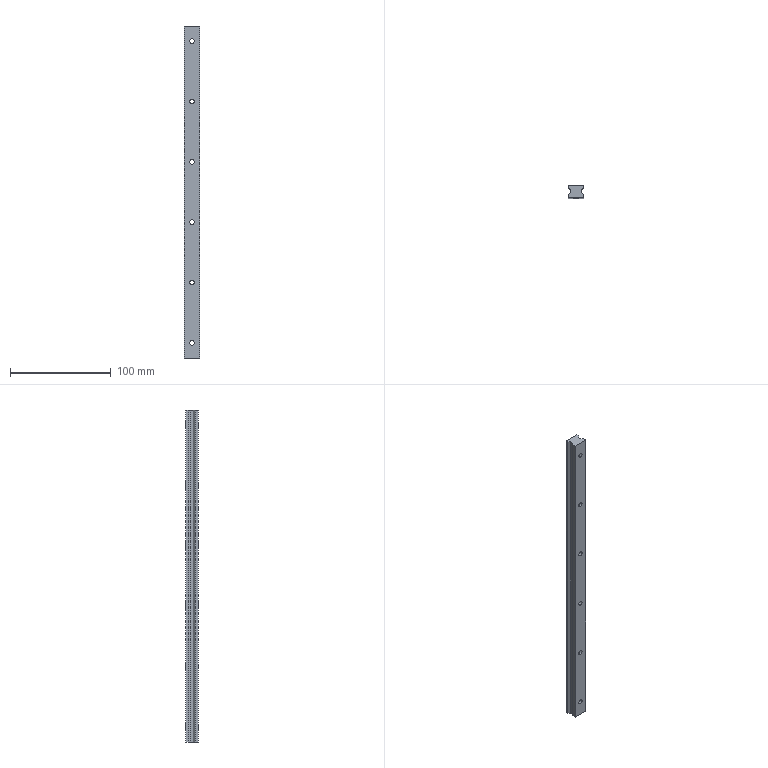Part | STEP file | 1 solid | 44 faces | box 15 x 12.5 x 330 mm | volume 52950 mm3 | cylinder 24 | plane 20 | commonest cylinder face diameters 4.5 x12 7.5 x12